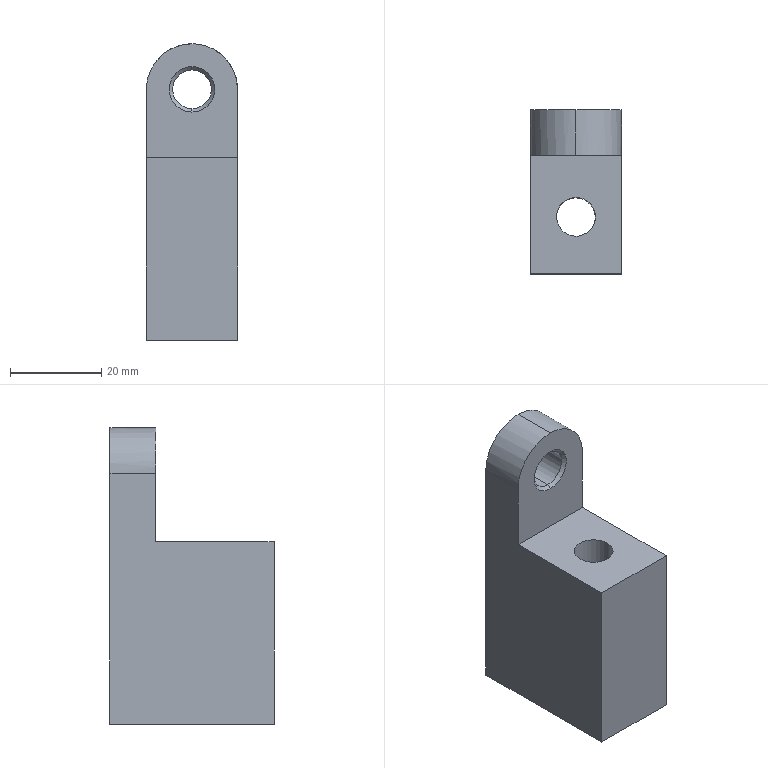Part | SolidWorks | features HoleWzd 3, BaseBody 1, Chamfer 1 | 1 solid | 21 faces | box 20 x 36.002 x 65.06 mm | volume 30270 mm3 | cylinder 8 | plane 7 | cone 6 | commonest cylinder face diameters 8.5 x4 6 x2 20 x2
STEP:
#1=CARTESIAN_POINT('',(406.077,357.037,79.285));
#2=VERTEX_POINT('',#1);
#3=CARTESIAN_POINT('',(406.077,357.037,87.785));
#4=VERTEX_POINT('',#3);
#5=CARTESIAN_POINT('',(406.077,357.037,83.535));
#6=DIRECTION('',(0.,1.,0.));
#7=DIRECTION('',(0.,0.,1.));
#8=AXIS2_PLACEMENT_3D('',#5,#6,#7);
#9=CIRCLE('',#8,4.25);
#10=EDGE_CURVE('',#2,#4,#9,.T.);
#11=ORIENTED_EDGE('',*,*,#10,.F.);
#12=CARTESIAN_POINT('',(406.077,357.787,78.535));
#13=VERTEX_POINT('',#12);
#14=CARTESIAN_POINT('',(406.077,357.037,79.285));
#15=DIRECTION('',(0.,0.7071,-0.7071));
#16=VECTOR('',#15,1000.);
#17=LINE('',#14,#16);
#18=EDGE_CURVE('',#2,#13,#17,.T.);
#19=ORIENTED_EDGE('',*,*,#18,.T.);
#20=CARTESIAN_POINT('',(406.077,357.787,88.535));
#21=VERTEX_POINT('',#20);
#22=CARTESIAN_POINT('',(406.077,357.787,83.535));
#23=DIRECTION('',(0.,-1.,0.));
#24=DIRECTION('',(0.,0.,1.));
#25=AXIS2_PLACEMENT_3D('',#22,#23,#24);
#26=CIRCLE('',#25,5.);
#27=EDGE_CURVE('',#21,#13,#26,.T.);
#28=ORIENTED_EDGE('',*,*,#27,.F.);
#29=CARTESIAN_POINT('',(406.077,357.037,87.785));
#30=DIRECTION('',(0.,0.7071,0.7071));
#31=VECTOR('',#30,1000.);
#32=LINE('',#29,#31);
#33=EDGE_CURVE('',#4,#21,#32,.T.);
#34=ORIENTED_EDGE('',*,*,#33,.F.);
#35=EDGE_LOOP('',(#11,#19,#28,#34));
#36=FACE_OUTER_BOUND('',#35,.T.);
#37=CARTESIAN_POINT('',(406.077,357.037,83.535));
#38=DIRECTION('',(0.,1.,0.));
#39=DIRECTION('',(0.,0.,1.));
#40=AXIS2_PLACEMENT_3D('',#37,#38,#39);
#41=CONICAL_SURFACE('',#40,4.25,0.7854);
#42=ADVANCED_FACE('',(#36),#41,.F.);
#43=CARTESIAN_POINT('',(406.077,348.537,87.785));
#44=VERTEX_POINT('',#43);
#45=CARTESIAN_POINT('',(406.077,348.537,79.285));
#46=VERTEX_POINT('',#45);
#47=CARTESIAN_POINT('',(406.077,348.537,83.535));
#48=DIRECTION('',(0.,-1.,0.));
#49=DIRECTION('',(0.,0.,1.));
#50=AXIS2_PLACEMENT_3D('',#47,#48,#49);
#51=CIRCLE('',#50,4.25);
#52=EDGE_CURVE('',#44,#46,#51,.T.);
#53=ORIENTED_EDGE('',*,*,#52,.F.);
#54=CARTESIAN_POINT('',(406.077,347.787,88.535));
#55=VERTEX_POINT('',#54);
#56=CARTESIAN_POINT('',(406.077,347.787,88.535));
#57=DIRECTION('',(0.,-0.7071,0.7071));
#58=VECTOR('',#57,1000.);
#59=LINE('',#56,#58);
#60=EDGE_CURVE('',#44,#55,#59,.T.);
#61=ORIENTED_EDGE('',*,*,#60,.T.);
#62=CARTESIAN_POINT('',(406.077,347.787,78.535));
#63=VERTEX_POINT('',#62);
#64=CARTESIAN_POINT('',(406.077,347.787,83.535));
#65=DIRECTION('',(0.,1.,0.));
#66=DIRECTION('',(0.,0.,1.));
#67=AXIS2_PLACEMENT_3D('',#64,#65,#66);
#68=CIRCLE('',#67,5.);
#69=EDGE_CURVE('',#63,#55,#68,.T.);
#70=ORIENTED_EDGE('',*,*,#69,.F.);
#71=CARTESIAN_POINT('',(406.077,347.787,78.535));
#72=DIRECTION('',(0.,-0.7071,-0.7071));
#73=VECTOR('',#72,1000.);
#74=LINE('',#71,#73);
#75=EDGE_CURVE('',#46,#63,#74,.T.);
#76=ORIENTED_EDGE('',*,*,#75,.F.);
#77=EDGE_LOOP('',(#53,#61,#70,#76));
#78=FACE_OUTER_BOUND('',#77,.T.);
#79=CARTESIAN_POINT('',(406.077,347.787,83.535));
#80=DIRECTION('',(0.,-1.,0.));
#81=DIRECTION('',(0.,0.,-1.));
#82=AXIS2_PLACEMENT_3D('',#79,#80,#81);
#83=CONICAL_SURFACE('',#82,5.,0.7854);
#84=ADVANCED_FACE('',(#78),#83,.F.);
#85=CARTESIAN_POINT('',(401.815,334.315,28.477));
#86=VERTEX_POINT('',#85);
#87=CARTESIAN_POINT('',(410.315,334.315,28.477));
#88=VERTEX_POINT('',#87);
#89=CARTESIAN_POINT('',(401.815,334.315,28.477));
#90=CARTESIAN_POINT('',(401.815,325.815,28.477));
#91=CARTESIAN_POINT('',(410.315,325.815,28.477));
#92=CARTESIAN_POINT('',(410.315,334.315,28.477));
#93=(BOUNDED_CURVE()B_SPLINE_CURVE(3,(#89,#90,#91,#92),.UNSPECIFIED.,.F.,.F.)B_SPLINE_CURVE_WITH_KNOTS((4,4),(3.605,6.747),.UNSPECIFIED.)CURVE()GEOMETRIC_REPRESENTATION_ITEM()RATIONAL_B_SPLINE_CURVE((1.,0.3333,0.3333,1.))REPRESENTATION_ITEM(''));
#94=EDGE_CURVE('',#86,#88,#93,.T.);
#95=ORIENTED_EDGE('',*,*,#94,.F.);
#96=CARTESIAN_POINT('',(401.827,334.31,68.539));
#97=VERTEX_POINT('',#96);
#98=CARTESIAN_POINT('',(401.827,334.31,68.542));
#99=DIRECTION('',(0.0002857,-0.0001428,1.));
#100=VECTOR('',#99,1000.);
#101=LINE('',#98,#100);
#102=EDGE_CURVE('',#86,#97,#101,.T.);
#103=ORIENTED_EDGE('',*,*,#102,.T.);
#104=CARTESIAN_POINT('',(410.327,334.31,68.539));
#105=VERTEX_POINT('',#104);
#106=CARTESIAN_POINT('',(401.827,334.31,68.539));
#107=CARTESIAN_POINT('',(401.827,325.81,68.54));
#108=CARTESIAN_POINT('',(410.327,325.81,68.54));
#109=CARTESIAN_POINT('',(410.327,334.31,68.539));
#110=(BOUNDED_CURVE()B_SPLINE_CURVE(3,(#106,#107,#108,#109),.UNSPECIFIED.,.F.,.F.)B_SPLINE_CURVE_WITH_KNOTS((4,4),(3.927,7.069),.UNSPECIFIED.)CURVE()GEOMETRIC_REPRESENTATION_ITEM()RATIONAL_B_SPLINE_CURVE((1.,0.3333,0.3333,1.))REPRESENTATION_ITEM(''));
#111=EDGE_CURVE('',#97,#105,#110,.T.);
#112=ORIENTED_EDGE('',*,*,#111,.T.);
#113=CARTESIAN_POINT('',(410.327,334.31,68.539));
#114=DIRECTION('',(0.0002857,-0.0001428,1.));
#115=VECTOR('',#114,1000.);
#116=LINE('',#113,#115);
#117=EDGE_CURVE('',#88,#105,#116,.T.);
#118=ORIENTED_EDGE('',*,*,#117,.F.);
#119=EDGE_LOOP('',(#95,#103,#112,#118));
#120=FACE_OUTER_BOUND('',#119,.T.);
#121=CARTESIAN_POINT('',(406.077,334.31,68.54));
#122=DIRECTION('',(0.0002857,-0.0001428,1.));
#123=DIRECTION('',(1.,0.,-0.0002857));
#124=AXIS2_PLACEMENT_3D('',#121,#122,#123);
#125=CYLINDRICAL_SURFACE('',#124,4.25);
#126=ADVANCED_FACE('',(#120),#125,.F.);
#127=CARTESIAN_POINT('',(409.071,348.177,38.477));
#128=VERTEX_POINT('',#127);
#129=CARTESIAN_POINT('',(403.071,348.177,38.477));
#130=VERTEX_POINT('',#129);
#131=CARTESIAN_POINT('',(406.071,348.177,38.477));
#132=DIRECTION('',(0.,0.,-1.));
#133=DIRECTION('',(-1.,0.,0.));
#134=AXIS2_PLACEMENT_3D('',#131,#132,#133);
#135=CIRCLE('',#134,3.);
#136=EDGE_CURVE('',#128,#130,#135,.T.);
#137=ORIENTED_EDGE('',*,*,#136,.F.);
#138=CARTESIAN_POINT('',(409.071,348.177,28.477));
#139=VERTEX_POINT('',#138);
#140=CARTESIAN_POINT('',(409.071,348.177,28.477));
#141=DIRECTION('',(0.,0.,-1.));
#142=VECTOR('',#141,1000.);
#143=LINE('',#140,#142);
#144=EDGE_CURVE('',#128,#139,#143,.T.);
#145=ORIENTED_EDGE('',*,*,#144,.T.);
#146=CARTESIAN_POINT('',(403.071,348.177,28.477));
#147=VERTEX_POINT('',#146);
#148=CARTESIAN_POINT('',(406.071,348.177,28.477));
#149=DIRECTION('',(0.,0.,-1.));
#150=DIRECTION('',(-1.,0.,0.));
#151=AXIS2_PLACEMENT_3D('',#148,#149,#150);
#152=CIRCLE('',#151,3.);
#153=EDGE_CURVE('',#139,#147,#152,.T.);
#154=ORIENTED_EDGE('',*,*,#153,.T.);
#155=CARTESIAN_POINT('',(403.071,348.177,28.477));
#156=DIRECTION('',(0.,0.,-1.));
#157=VECTOR('',#156,1000.);
#158=LINE('',#155,#157);
#159=EDGE_CURVE('',#130,#147,#158,.T.);
#160=ORIENTED_EDGE('',*,*,#159,.F.);
#161=EDGE_LOOP('',(#137,#145,#154,#160));
#162=FACE_OUTER_BOUND('',#161,.T.);
#163=CARTESIAN_POINT('',(406.071,348.177,28.477));
#164=DIRECTION('',(0.,0.,-1.));
#165=DIRECTION('',(-1.,0.,0.));
#166=AXIS2_PLACEMENT_3D('',#163,#164,#165);
#167=CYLINDRICAL_SURFACE('',#166,3.);
#168=ADVANCED_FACE('',(#162),#167,.F.);
#169=CARTESIAN_POINT('',(406.071,348.177,39.28));
#170=VERTEX_POINT('',#169);
#171=CARTESIAN_POINT('',(403.071,348.177,38.477));
#172=DIRECTION('',(-0.9659,0.,-0.2588));
#173=VECTOR('',#172,1000.);
#174=LINE('',#171,#173);
#175=EDGE_CURVE('',#170,#130,#174,.T.);
#176=ORIENTED_EDGE('',*,*,#175,.F.);
#177=CARTESIAN_POINT('',(409.071,348.177,38.477));
#178=DIRECTION('',(0.9659,0.,-0.2588));
#179=VECTOR('',#178,1000.);
#180=LINE('',#177,#179);
#181=EDGE_CURVE('',#170,#128,#180,.T.);
#182=ORIENTED_EDGE('',*,*,#181,.T.);
#183=ORIENTED_EDGE('',*,*,#136,.T.);
#184=EDGE_LOOP('',(#176,#182,#183));
#185=FACE_OUTER_BOUND('',#184,.T.);
#186=CARTESIAN_POINT('',(406.071,348.177,38.477));
#187=DIRECTION('',(0.,0.,-1.));
#188=DIRECTION('',(-1.,0.,0.));
#189=AXIS2_PLACEMENT_3D('',#186,#187,#188);
#190=CONICAL_SURFACE('',#189,3.,1.309);
#191=ADVANCED_FACE('',(#185),#190,.F.);
#192=ORIENTED_EDGE('',*,*,#52,.T.);
#193=CARTESIAN_POINT('',(406.077,357.787,79.285));
#194=DIRECTION('',(0.,1.,0.));
#195=VECTOR('',#194,1000.);
#196=LINE('',#193,#195);
#197=EDGE_CURVE('',#46,#2,#196,.T.);
#198=ORIENTED_EDGE('',*,*,#197,.T.);
#199=ORIENTED_EDGE('',*,*,#10,.T.);
#200=CARTESIAN_POINT('',(406.077,357.787,87.785));
#201=DIRECTION('',(0.,1.,0.));
#202=VECTOR('',#201,1000.);
#203=LINE('',#200,#202);
#204=EDGE_CURVE('',#44,#4,#203,.T.);
#205=ORIENTED_EDGE('',*,*,#204,.F.);
#206=EDGE_LOOP('',(#192,#198,#199,#205));
#207=FACE_OUTER_BOUND('',#206,.T.);
#208=CARTESIAN_POINT('',(406.077,357.787,83.535));
#209=DIRECTION('',(0.,1.,0.));
#210=DIRECTION('',(0.,0.,1.));
#211=AXIS2_PLACEMENT_3D('',#208,#209,#210);
#212=CYLINDRICAL_SURFACE('',#211,4.25);
#213=ADVANCED_FACE('',(#207),#212,.F.);
#214=CARTESIAN_POINT('',(406.077,347.787,93.537));
#215=VERTEX_POINT('',#214);
#216=CARTESIAN_POINT('',(396.077,347.787,83.538));
#217=VERTEX_POINT('',#216);
#218=CARTESIAN_POINT('',(406.077,347.787,93.537));
#219=CARTESIAN_POINT('',(400.22,347.787,93.537));
#220=CARTESIAN_POINT('',(396.078,347.787,89.395));
#221=CARTESIAN_POINT('',(396.077,347.787,83.538));
#222=(BOUNDED_CURVE()B_SPLINE_CURVE(3,(#218,#219,#220,#221),.UNSPECIFIED.,.F.,.F.)B_SPLINE_CURVE_WITH_KNOTS((4,4),(3.142,4.713),.UNSPECIFIED.)CURVE()GEOMETRIC_REPRESENTATION_ITEM()RATIONAL_B_SPLINE_CURVE((1.,0.8048,0.8048,1.))REPRESENTATION_ITEM(''));
#223=EDGE_CURVE('',#215,#217,#222,.T.);
#224=ORIENTED_EDGE('',*,*,#223,.F.);
#225=CARTESIAN_POINT('',(406.077,357.787,93.535));
#226=VERTEX_POINT('',#225);
#227=CARTESIAN_POINT('',(406.077,334.796,93.539));
#228=DIRECTION('',(-0.000000041,1.,-0.0001428));
#229=VECTOR('',#228,1000.);
#230=LINE('',#227,#229);
#231=EDGE_CURVE('',#215,#226,#230,.T.);
#232=ORIENTED_EDGE('',*,*,#231,.T.);
#233=CARTESIAN_POINT('',(396.077,357.787,83.536));
#234=VERTEX_POINT('',#233);
#235=CARTESIAN_POINT('',(396.077,357.787,83.536));
#236=CARTESIAN_POINT('',(396.078,357.787,89.394));
#237=CARTESIAN_POINT('',(400.22,357.787,93.535));
#238=CARTESIAN_POINT('',(406.077,357.787,93.535));
#239=(BOUNDED_CURVE()B_SPLINE_CURVE(3,(#235,#236,#237,#238),.UNSPECIFIED.,.F.,.F.)B_SPLINE_CURVE_WITH_KNOTS((4,4),(1.571,3.141),.UNSPECIFIED.)CURVE()GEOMETRIC_REPRESENTATION_ITEM()RATIONAL_B_SPLINE_CURVE((1.,0.8048,0.8048,1.))REPRESENTATION_ITEM(''));
#240=EDGE_CURVE('',#234,#226,#239,.T.);
#241=ORIENTED_EDGE('',*,*,#240,.F.);
#242=CARTESIAN_POINT('',(396.077,357.787,83.536));
#243=DIRECTION('',(0.000000041,-1.,0.0001428));
#244=VECTOR('',#243,1000.);
#245=LINE('',#242,#244);
#246=EDGE_CURVE('',#234,#217,#245,.T.);
#247=ORIENTED_EDGE('',*,*,#246,.T.);
#248=EDGE_LOOP('',(#224,#232,#241,#247));
#249=FACE_OUTER_BOUND('',#248,.T.);
#250=CARTESIAN_POINT('',(406.077,334.795,83.539));
#251=DIRECTION('',(-0.000000041,1.,-0.0001428));
#252=DIRECTION('',(0.,0.0001428,1.));
#253=AXIS2_PLACEMENT_3D('',#250,#251,#252);
#254=CYLINDRICAL_SURFACE('',#253,10.);
#255=ADVANCED_FACE('',(#249),#254,.T.);
#256=CARTESIAN_POINT('',(396.077,321.784,28.477));
#257=VERTEX_POINT('',#256);
#258=CARTESIAN_POINT('',(396.077,321.784,68.54));
#259=VERTEX_POINT('',#258);
#260=CARTESIAN_POINT('',(396.077,321.784,28.477));
#261=DIRECTION('',(0.,0.,1.));
#262=VECTOR('',#261,1000.);
#263=LINE('',#260,#262);
#264=EDGE_CURVE('',#257,#259,#263,.T.);
#265=ORIENTED_EDGE('',*,*,#264,.F.);
#266=CARTESIAN_POINT('',(416.077,321.784,28.477));
#267=VERTEX_POINT('',#266);
#268=CARTESIAN_POINT('',(416.077,321.784,28.477));
#269=DIRECTION('',(-1.,0.,0.));
#270=VECTOR('',#269,1000.);
#271=LINE('',#268,#270);
#272=EDGE_CURVE('',#267,#257,#271,.T.);
#273=ORIENTED_EDGE('',*,*,#272,.F.);
#274=CARTESIAN_POINT('',(416.077,321.784,68.54));
#275=VERTEX_POINT('',#274);
#276=CARTESIAN_POINT('',(416.077,321.784,68.54));
#277=DIRECTION('',(0.,0.,-1.));
#278=VECTOR('',#277,1000.);
#279=LINE('',#276,#278);
#280=EDGE_CURVE('',#275,#267,#279,.T.);
#281=ORIENTED_EDGE('',*,*,#280,.F.);
#282=CARTESIAN_POINT('',(396.077,321.784,68.54));
#283=DIRECTION('',(1.,0.,0.));
#284=VECTOR('',#283,1000.);
#285=LINE('',#282,#284);
#286=EDGE_CURVE('',#259,#275,#285,.T.);
#287=ORIENTED_EDGE('',*,*,#286,.F.);
#288=EDGE_LOOP('',(#265,#273,#281,#287));
#289=FACE_OUTER_BOUND('',#288,.T.);
#290=CARTESIAN_POINT('',(405.902,321.784,18.477));
#291=DIRECTION('',(0.,-1.,0.));
#292=DIRECTION('',(0.,0.,-1.));
#293=AXIS2_PLACEMENT_3D('',#290,#291,#292);
#294=PLANE('',#293);
#295=ADVANCED_FACE('',(#289),#294,.T.);
#296=ORIENTED_EDGE('',*,*,#231,.F.);
#297=CARTESIAN_POINT('',(416.077,347.787,83.536));
#298=VERTEX_POINT('',#297);
#299=CARTESIAN_POINT('',(416.077,347.787,83.536));
#300=CARTESIAN_POINT('',(416.078,347.787,89.394));
#301=CARTESIAN_POINT('',(411.936,347.787,93.537));
#302=CARTESIAN_POINT('',(406.077,347.787,93.537));
#303=(BOUNDED_CURVE()B_SPLINE_CURVE(3,(#299,#300,#301,#302),.UNSPECIFIED.,.F.,.F.)B_SPLINE_CURVE_WITH_KNOTS((4,4),(1.571,3.142),.UNSPECIFIED.)CURVE()GEOMETRIC_REPRESENTATION_ITEM()RATIONAL_B_SPLINE_CURVE((1.,0.8047,0.8047,1.))REPRESENTATION_ITEM(''));
#304=EDGE_CURVE('',#298,#215,#303,.T.);
#305=ORIENTED_EDGE('',*,*,#304,.F.);
#306=CARTESIAN_POINT('',(416.077,357.787,83.534));
#307=VERTEX_POINT('',#306);
#308=CARTESIAN_POINT('',(416.077,347.787,83.536));
#309=DIRECTION('',(-0.000000041,1.,-0.0001428));
#310=VECTOR('',#309,1000.);
#311=LINE('',#308,#310);
#312=EDGE_CURVE('',#298,#307,#311,.T.);
#313=ORIENTED_EDGE('',*,*,#312,.T.);
#314=CARTESIAN_POINT('',(406.077,357.787,93.535));
#315=CARTESIAN_POINT('',(411.936,357.787,93.535));
#316=CARTESIAN_POINT('',(416.078,357.787,89.393));
#317=CARTESIAN_POINT('',(416.077,357.787,83.534));
#318=(BOUNDED_CURVE()B_SPLINE_CURVE(3,(#314,#315,#316,#317),.UNSPECIFIED.,.F.,.F.)B_SPLINE_CURVE_WITH_KNOTS((4,4),(3.141,4.712),.UNSPECIFIED.)CURVE()GEOMETRIC_REPRESENTATION_ITEM()RATIONAL_B_SPLINE_CURVE((1.,0.8047,0.8047,1.))REPRESENTATION_ITEM(''));
#319=EDGE_CURVE('',#226,#307,#318,.T.);
#320=ORIENTED_EDGE('',*,*,#319,.F.);
#321=EDGE_LOOP('',(#296,#305,#313,#320));
#322=FACE_OUTER_BOUND('',#321,.T.);
#323=CARTESIAN_POINT('',(406.077,334.795,83.539));
#324=DIRECTION('',(-0.000000041,1.,-0.0001428));
#325=DIRECTION('',(0.,0.0001428,1.));
#326=AXIS2_PLACEMENT_3D('',#323,#324,#325);
#327=CYLINDRICAL_SURFACE('',#326,10.);
#328=ADVANCED_FACE('',(#322),#327,.T.);
#329=ORIENTED_EDGE('',*,*,#27,.T.);
#330=CARTESIAN_POINT('',(406.077,357.787,83.535));
#331=DIRECTION('',(0.,-1.,0.));
#332=DIRECTION('',(0.,0.,1.));
#333=AXIS2_PLACEMENT_3D('',#330,#331,#332);
#334=CIRCLE('',#333,5.);
#335=EDGE_CURVE('',#13,#21,#334,.T.);
#336=ORIENTED_EDGE('',*,*,#335,.T.);
#337=EDGE_LOOP('',(#329,#336));
#338=FACE_BOUND('',#337,.T.);
#339=CARTESIAN_POINT('',(396.077,357.787,28.477));
#340=VERTEX_POINT('',#339);
#341=CARTESIAN_POINT('',(396.077,357.787,83.536));
#342=DIRECTION('',(0.,-0.000000007,-1.));
#343=VECTOR('',#342,1000.);
#344=LINE('',#341,#343);
#345=EDGE_CURVE('',#234,#340,#344,.T.);
#346=ORIENTED_EDGE('',*,*,#345,.F.);
#347=ORIENTED_EDGE('',*,*,#240,.T.);
#348=ORIENTED_EDGE('',*,*,#319,.T.);
#349=CARTESIAN_POINT('',(416.077,357.787,28.477));
#350=VERTEX_POINT('',#349);
#351=CARTESIAN_POINT('',(416.077,357.787,83.534));
#352=DIRECTION('',(0.,0.000000007,-1.));
#353=VECTOR('',#352,1000.);
#354=LINE('',#351,#353);
#355=EDGE_CURVE('',#307,#350,#354,.T.);
#356=ORIENTED_EDGE('',*,*,#355,.T.);
#357=CARTESIAN_POINT('',(416.077,357.787,28.477));
#358=DIRECTION('',(-1.,0.,0.));
#359=VECTOR('',#358,1000.);
#360=LINE('',#357,#359);
#361=EDGE_CURVE('',#350,#340,#360,.T.);
#362=ORIENTED_EDGE('',*,*,#361,.T.);
#363=EDGE_LOOP('',(#346,#347,#348,#356,#362));
#364=FACE_OUTER_BOUND('',#363,.T.);
#365=CARTESIAN_POINT('',(405.902,357.787,18.477));
#366=DIRECTION('',(0.,1.,0.));
#367=DIRECTION('',(1.,0.,0.));
#368=AXIS2_PLACEMENT_3D('',#365,#366,#367);
#369=PLANE('',#368);
#370=ADVANCED_FACE('',(#338,#364),#369,.T.);
#371=ORIENTED_EDGE('',*,*,#264,.T.);
#372=CARTESIAN_POINT('',(396.077,347.787,68.537));
#373=VERTEX_POINT('',#372);
#374=CARTESIAN_POINT('',(396.077,347.787,68.537));
#375=DIRECTION('',(0.000000041,-1.,0.0001428));
#376=VECTOR('',#375,1000.);
#377=LINE('',#374,#376);
#378=EDGE_CURVE('',#373,#259,#377,.T.);
#379=ORIENTED_EDGE('',*,*,#378,.F.);
#380=CARTESIAN_POINT('',(396.077,347.787,83.538));
#381=DIRECTION('',(0.,-0.000000025,-1.));
#382=VECTOR('',#381,1000.);
#383=LINE('',#380,#382);
#384=EDGE_CURVE('',#217,#373,#383,.T.);
#385=ORIENTED_EDGE('',*,*,#384,.F.);
#386=ORIENTED_EDGE('',*,*,#246,.F.);
#387=ORIENTED_EDGE('',*,*,#345,.T.);
#388=CARTESIAN_POINT('',(396.077,357.787,28.477));
#389=DIRECTION('',(0.000000041,-1.,0.));
#390=VECTOR('',#389,1000.);
#391=LINE('',#388,#390);
#392=EDGE_CURVE('',#340,#257,#391,.T.);
#393=ORIENTED_EDGE('',*,*,#392,.T.);
#394=EDGE_LOOP('',(#371,#379,#385,#386,#387,#393));
#395=FACE_OUTER_BOUND('',#394,.T.);
#396=CARTESIAN_POINT('',(396.077,334.785,18.477));
#397=DIRECTION('',(-1.,-0.000000041,0.));
#398=DIRECTION('',(-0.000000041,1.,0.));
#399=AXIS2_PLACEMENT_3D('',#396,#397,#398);
#400=PLANE('',#399);
#401=ADVANCED_FACE('',(#395),#400,.T.);
#402=CARTESIAN_POINT('',(410.327,334.31,68.539));
#403=CARTESIAN_POINT('',(410.327,342.81,68.537));
#404=CARTESIAN_POINT('',(401.827,342.81,68.537));
#405=CARTESIAN_POINT('',(401.827,334.31,68.539));
#406=(BOUNDED_CURVE()B_SPLINE_CURVE(3,(#402,#403,#404,#405),.UNSPECIFIED.,.F.,.F.)B_SPLINE_CURVE_WITH_KNOTS((4,4),(0.7854,3.927),.UNSPECIFIED.)CURVE()GEOMETRIC_REPRESENTATION_ITEM()RATIONAL_B_SPLINE_CURVE((1.,0.3333,0.3333,1.))REPRESENTATION_ITEM(''));
#407=EDGE_CURVE('',#105,#97,#406,.T.);
#408=ORIENTED_EDGE('',*,*,#407,.F.);
#409=ORIENTED_EDGE('',*,*,#111,.F.);
#410=EDGE_LOOP('',(#408,#409));
#411=FACE_BOUND('',#410,.T.);
#412=ORIENTED_EDGE('',*,*,#286,.T.);
#413=CARTESIAN_POINT('',(416.077,347.787,68.537));
#414=VERTEX_POINT('',#413);
#415=CARTESIAN_POINT('',(416.077,321.784,68.54));
#416=DIRECTION('',(-0.000000041,1.,-0.0001428));
#417=VECTOR('',#416,1000.);
#418=LINE('',#415,#417);
#419=EDGE_CURVE('',#275,#414,#418,.T.);
#420=ORIENTED_EDGE('',*,*,#419,.T.);
#421=CARTESIAN_POINT('',(396.077,347.787,68.537));
#422=DIRECTION('',(1.,0.,0.));
#423=VECTOR('',#422,1000.);
#424=LINE('',#421,#423);
#425=EDGE_CURVE('',#373,#414,#424,.T.);
#426=ORIENTED_EDGE('',*,*,#425,.F.);
#427=ORIENTED_EDGE('',*,*,#378,.T.);
#428=EDGE_LOOP('',(#412,#420,#426,#427));
#429=FACE_OUTER_BOUND('',#428,.T.);
#430=CARTESIAN_POINT('',(405.902,334.789,68.539));
#431=DIRECTION('',(0.,0.0001428,1.));
#432=DIRECTION('',(1.,0.000000041,0.));
#433=AXIS2_PLACEMENT_3D('',#430,#431,#432);
#434=PLANE('',#433);
#435=ADVANCED_FACE('',(#411,#429),#434,.T.);
#436=CARTESIAN_POINT('',(410.315,334.315,28.477));
#437=CARTESIAN_POINT('',(410.315,342.815,28.477));
#438=CARTESIAN_POINT('',(401.815,342.815,28.477));
#439=CARTESIAN_POINT('',(401.815,334.315,28.477));
#440=(BOUNDED_CURVE()B_SPLINE_CURVE(3,(#436,#437,#438,#439),.UNSPECIFIED.,.F.,.F.)B_SPLINE_CURVE_WITH_KNOTS((4,4),(0.4636,3.605),.UNSPECIFIED.)CURVE()GEOMETRIC_REPRESENTATION_ITEM()RATIONAL_B_SPLINE_CURVE((1.,0.3333,0.3333,1.))REPRESENTATION_ITEM(''));
#441=EDGE_CURVE('',#88,#86,#440,.T.);
#442=ORIENTED_EDGE('',*,*,#441,.T.);
#443=ORIENTED_EDGE('',*,*,#94,.T.);
#444=EDGE_LOOP('',(#442,#443));
#445=FACE_BOUND('',#444,.T.);
#446=CARTESIAN_POINT('',(406.071,348.177,28.477));
#447=DIRECTION('',(0.,0.,-1.));
#448=DIRECTION('',(-1.,0.,0.));
#449=AXIS2_PLACEMENT_3D('',#446,#447,#448);
#450=CIRCLE('',#449,3.);
#451=EDGE_CURVE('',#147,#139,#450,.T.);
#452=ORIENTED_EDGE('',*,*,#451,.F.);
#453=ORIENTED_EDGE('',*,*,#153,.F.);
#454=EDGE_LOOP('',(#452,#453));
#455=FACE_BOUND('',#454,.T.);
#456=ORIENTED_EDGE('',*,*,#361,.F.);
#457=CARTESIAN_POINT('',(416.077,321.784,28.477));
#458=DIRECTION('',(-0.000000041,1.,0.));
#459=VECTOR('',#458,1000.);
#460=LINE('',#457,#459);
#461=EDGE_CURVE('',#267,#350,#460,.T.);
#462=ORIENTED_EDGE('',*,*,#461,.F.);
#463=ORIENTED_EDGE('',*,*,#272,.T.);
#464=ORIENTED_EDGE('',*,*,#392,.F.);
#465=EDGE_LOOP('',(#456,#462,#463,#464));
#466=FACE_OUTER_BOUND('',#465,.T.);
#467=CARTESIAN_POINT('',(411.172,260.65,28.477));
#468=DIRECTION('',(0.,0.,1.));
#469=DIRECTION('',(1.,0.,0.));
#470=AXIS2_PLACEMENT_3D('',#467,#468,#469);
#471=PLANE('',#470);
#472=ADVANCED_FACE('',(#445,#455,#466),#471,.F.);
#473=ORIENTED_EDGE('',*,*,#355,.F.);
#474=ORIENTED_EDGE('',*,*,#312,.F.);
#475=CARTESIAN_POINT('',(416.077,347.787,68.537));
#476=DIRECTION('',(0.,-0.000000025,1.));
#477=VECTOR('',#476,1000.);
#478=LINE('',#475,#477);
#479=EDGE_CURVE('',#414,#298,#478,.T.);
#480=ORIENTED_EDGE('',*,*,#479,.F.);
#481=ORIENTED_EDGE('',*,*,#419,.F.);
#482=ORIENTED_EDGE('',*,*,#280,.T.);
#483=ORIENTED_EDGE('',*,*,#461,.T.);
#484=EDGE_LOOP('',(#473,#474,#480,#481,#482,#483));
#485=FACE_OUTER_BOUND('',#484,.T.);
#486=CARTESIAN_POINT('',(416.077,334.785,18.477));
#487=DIRECTION('',(1.,0.000000041,0.));
#488=DIRECTION('',(0.,-0.0001428,-1.));
#489=AXIS2_PLACEMENT_3D('',#486,#487,#488);
#490=PLANE('',#489);
#491=ADVANCED_FACE('',(#485),#490,.T.);
#492=ORIENTED_EDGE('',*,*,#69,.T.);
#493=CARTESIAN_POINT('',(406.077,347.787,83.535));
#494=DIRECTION('',(0.,1.,0.));
#495=DIRECTION('',(0.,0.,1.));
#496=AXIS2_PLACEMENT_3D('',#493,#494,#495);
#497=CIRCLE('',#496,5.);
#498=EDGE_CURVE('',#55,#63,#497,.T.);
#499=ORIENTED_EDGE('',*,*,#498,.T.);
#500=EDGE_LOOP('',(#492,#499));
#501=FACE_BOUND('',#500,.T.);
#502=ORIENTED_EDGE('',*,*,#304,.T.);
#503=ORIENTED_EDGE('',*,*,#223,.T.);
#504=ORIENTED_EDGE('',*,*,#384,.T.);
#505=ORIENTED_EDGE('',*,*,#425,.T.);
#506=ORIENTED_EDGE('',*,*,#479,.T.);
#507=EDGE_LOOP('',(#502,#503,#504,#505,#506));
#508=FACE_OUTER_BOUND('',#507,.T.);
#509=CARTESIAN_POINT('',(405.902,347.787,32.007));
#510=DIRECTION('',(0.,1.,0.));
#511=DIRECTION('',(1.,0.,0.));
#512=AXIS2_PLACEMENT_3D('',#509,#510,#511);
#513=PLANE('',#512);
#514=ADVANCED_FACE('',(#501,#508),#513,.F.);
#515=ORIENTED_EDGE('',*,*,#197,.F.);
#516=CARTESIAN_POINT('',(406.077,348.537,83.535));
#517=DIRECTION('',(0.,-1.,0.));
#518=DIRECTION('',(0.,0.,1.));
#519=AXIS2_PLACEMENT_3D('',#516,#517,#518);
#520=CIRCLE('',#519,4.25);
#521=EDGE_CURVE('',#46,#44,#520,.T.);
#522=ORIENTED_EDGE('',*,*,#521,.T.);
#523=ORIENTED_EDGE('',*,*,#204,.T.);
#524=CARTESIAN_POINT('',(406.077,357.037,83.535));
#525=DIRECTION('',(0.,1.,0.));
#526=DIRECTION('',(0.,0.,1.));
#527=AXIS2_PLACEMENT_3D('',#524,#525,#526);
#528=CIRCLE('',#527,4.25);
#529=EDGE_CURVE('',#4,#2,#528,.T.);
#530=ORIENTED_EDGE('',*,*,#529,.T.);
#531=EDGE_LOOP('',(#515,#522,#523,#530));
#532=FACE_OUTER_BOUND('',#531,.T.);
#533=CARTESIAN_POINT('',(406.077,357.787,83.535));
#534=DIRECTION('',(0.,1.,0.));
#535=DIRECTION('',(0.,0.,1.));
#536=AXIS2_PLACEMENT_3D('',#533,#534,#535);
#537=CYLINDRICAL_SURFACE('',#536,4.25);
#538=ADVANCED_FACE('',(#532),#537,.F.);
#539=ORIENTED_EDGE('',*,*,#181,.F.);
#540=ORIENTED_EDGE('',*,*,#175,.T.);
#541=CARTESIAN_POINT('',(406.071,348.177,38.477));
#542=DIRECTION('',(0.,0.,-1.));
#543=DIRECTION('',(-1.,0.,0.));
#544=AXIS2_PLACEMENT_3D('',#541,#542,#543);
#545=CIRCLE('',#544,3.);
#546=EDGE_CURVE('',#130,#128,#545,.T.);
#547=ORIENTED_EDGE('',*,*,#546,.T.);
#548=EDGE_LOOP('',(#539,#540,#547));
#549=FACE_OUTER_BOUND('',#548,.T.);
#550=CARTESIAN_POINT('',(406.071,348.177,38.477));
#551=DIRECTION('',(0.,0.,-1.));
#552=DIRECTION('',(-1.,0.,0.));
#553=AXIS2_PLACEMENT_3D('',#550,#551,#552);
#554=CONICAL_SURFACE('',#553,3.,1.309);
#555=ADVANCED_FACE('',(#549),#554,.F.);
#556=ORIENTED_EDGE('',*,*,#144,.F.);
#557=ORIENTED_EDGE('',*,*,#546,.F.);
#558=ORIENTED_EDGE('',*,*,#159,.T.);
#559=ORIENTED_EDGE('',*,*,#451,.T.);
#560=EDGE_LOOP('',(#556,#557,#558,#559));
#561=FACE_OUTER_BOUND('',#560,.T.);
#562=CARTESIAN_POINT('',(406.071,348.177,28.477));
#563=DIRECTION('',(0.,0.,-1.));
#564=DIRECTION('',(-1.,0.,0.));
#565=AXIS2_PLACEMENT_3D('',#562,#563,#564);
#566=CYLINDRICAL_SURFACE('',#565,3.);
#567=ADVANCED_FACE('',(#561),#566,.F.);
#568=ORIENTED_EDGE('',*,*,#102,.F.);
#569=ORIENTED_EDGE('',*,*,#441,.F.);
#570=ORIENTED_EDGE('',*,*,#117,.T.);
#571=ORIENTED_EDGE('',*,*,#407,.T.);
#572=EDGE_LOOP('',(#568,#569,#570,#571));
#573=FACE_OUTER_BOUND('',#572,.T.);
#574=CARTESIAN_POINT('',(406.077,334.31,68.54));
#575=DIRECTION('',(0.0002857,-0.0001428,1.));
#576=DIRECTION('',(1.,0.,-0.0002857));
#577=AXIS2_PLACEMENT_3D('',#574,#575,#576);
#578=CYLINDRICAL_SURFACE('',#577,4.25);
#579=ADVANCED_FACE('',(#573),#578,.F.);
#580=ORIENTED_EDGE('',*,*,#60,.F.);
#581=ORIENTED_EDGE('',*,*,#521,.F.);
#582=ORIENTED_EDGE('',*,*,#75,.T.);
#583=ORIENTED_EDGE('',*,*,#498,.F.);
#584=EDGE_LOOP('',(#580,#581,#582,#583));
#585=FACE_OUTER_BOUND('',#584,.T.);
#586=CARTESIAN_POINT('',(406.077,347.787,83.535));
#587=DIRECTION('',(0.,-1.,0.));
#588=DIRECTION('',(0.,0.,-1.));
#589=AXIS2_PLACEMENT_3D('',#586,#587,#588);
#590=CONICAL_SURFACE('',#589,5.,0.7854);
#591=ADVANCED_FACE('',(#585),#590,.F.);
#592=ORIENTED_EDGE('',*,*,#18,.F.);
#593=ORIENTED_EDGE('',*,*,#529,.F.);
#594=ORIENTED_EDGE('',*,*,#33,.T.);
#595=ORIENTED_EDGE('',*,*,#335,.F.);
#596=EDGE_LOOP('',(#592,#593,#594,#595));
#597=FACE_OUTER_BOUND('',#596,.T.);
#598=CARTESIAN_POINT('',(406.077,357.037,83.535));
#599=DIRECTION('',(0.,1.,0.));
#600=DIRECTION('',(0.,0.,1.));
#601=AXIS2_PLACEMENT_3D('',#598,#599,#600);
#602=CONICAL_SURFACE('',#601,4.25,0.7854);
#603=ADVANCED_FACE('',(#597),#602,.F.);
#604=CLOSED_SHELL('',(#42,#84,#126,#168,#191,#213,#255,#295,#328,#370,#401,#435,#472,#491,#514,#538,#555,#567,#579,#591,#603));
#605=MANIFOLD_SOLID_BREP('',#604);
#606=CARTESIAN_POINT('',(0.,0.,0.));
#607=DIRECTION('',(0.,0.,1.));
#608=DIRECTION('',(1.,0.,0.));
#609=AXIS2_PLACEMENT_3D('',#606,#607,#608);
#610=(LENGTH_UNIT()NAMED_UNIT(*)SI_UNIT(.MILLI.,.METRE.));
#611=UNCERTAINTY_MEASURE_WITH_UNIT(LENGTH_MEASURE(0.00001),#610,'','');
#612=(NAMED_UNIT(*)PLANE_ANGLE_UNIT()SI_UNIT($,.RADIAN.));
#613=(NAMED_UNIT(*)SI_UNIT($,.STERADIAN.)SOLID_ANGLE_UNIT());
#614=(GEOMETRIC_REPRESENTATION_CONTEXT(3)GLOBAL_UNCERTAINTY_ASSIGNED_CONTEXT((#611))GLOBAL_UNIT_ASSIGNED_CONTEXT((#610,#612,#613))REPRESENTATION_CONTEXT('',''));
#615=ADVANCED_BREP_SHAPE_REPRESENTATION('',(#605,#609),#614);